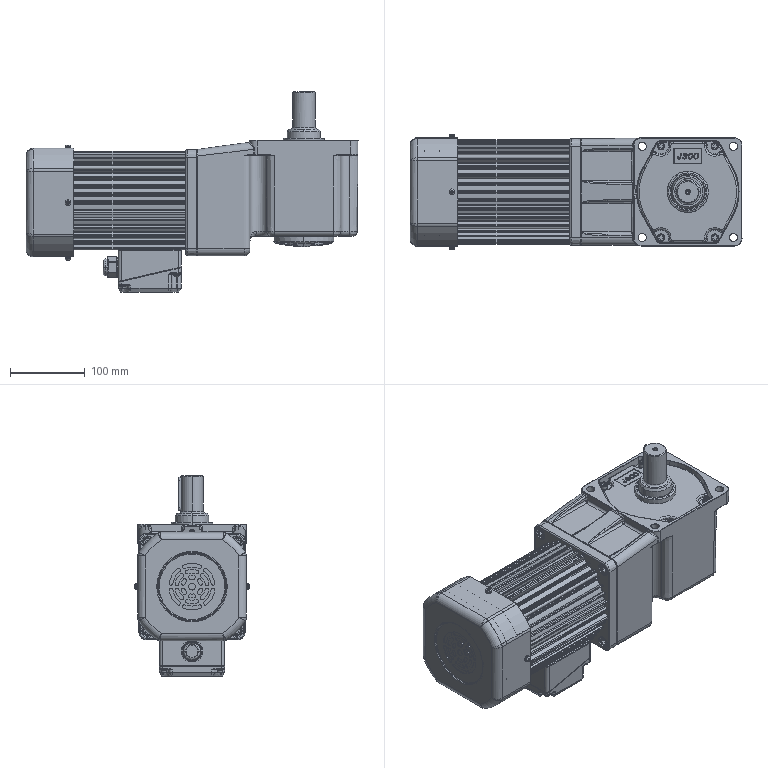Part | SolidWorks | 4 solids | 3393 faces | volume 5746372 mm3 | cylinder 1167 | plane 904 | spline 865 | torus 352 | cone 80 | sphere 25 | commonest cylinder face diameters 2 x182 0.4 x158 4 x124 1 x113 3 x47 8 x47